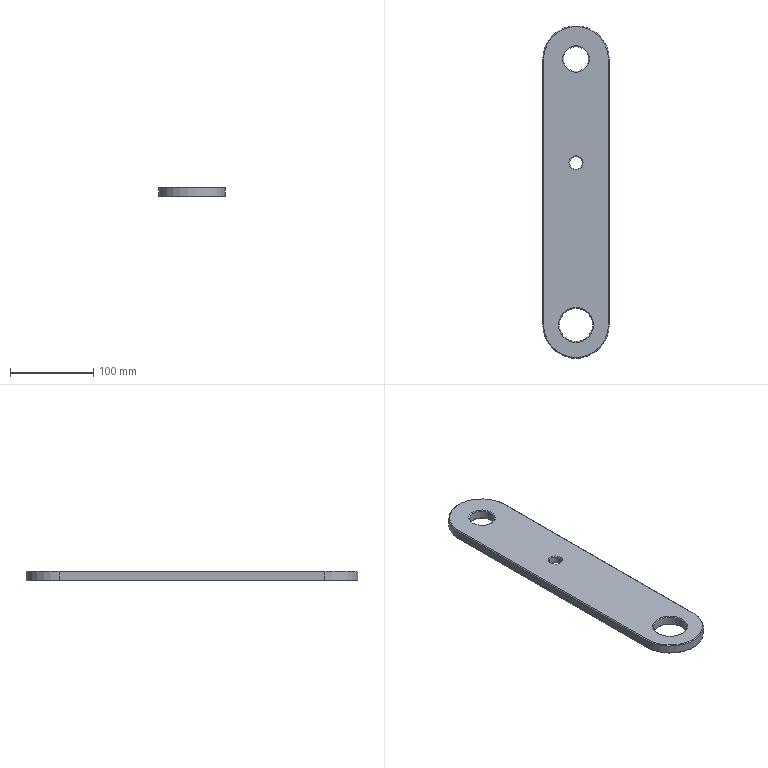Part | SolidWorks | features BaseBody 1 | 1 solid | 35 faces | box 80 x 400 x 12 mm | volume 339060 mm3 | cone 16 | cylinder 10 | plane 9 | commonest cylinder face diameters 30 x4 15 x2 40 x2 80 x2
STEP:
#1=CARTESIAN_POINT('',(-20.,-320.,11.));
#2=VERTEX_POINT('',#1);
#3=CARTESIAN_POINT('',(-21.,-320.,12.));
#4=VERTEX_POINT('',#3);
#5=CARTESIAN_POINT('',(-20.,-320.,11.));
#6=DIRECTION('',(-0.7071,0.,0.7071));
#7=VECTOR('',#6,1000.);
#8=LINE('',#5,#7);
#9=EDGE_CURVE('',#2,#4,#8,.T.);
#10=ORIENTED_EDGE('',*,*,#9,.F.);
#11=CARTESIAN_POINT('',(20.,-320.,11.));
#12=VERTEX_POINT('',#11);
#13=CARTESIAN_POINT('',(0.,-320.,11.));
#14=DIRECTION('',(0.,0.,1.));
#15=DIRECTION('',(1.,0.,0.));
#16=AXIS2_PLACEMENT_3D('',#13,#14,#15);
#17=CIRCLE('',#16,20.);
#18=EDGE_CURVE('',#12,#2,#17,.T.);
#19=ORIENTED_EDGE('',*,*,#18,.F.);
#20=CARTESIAN_POINT('',(21.,-320.,12.));
#21=VERTEX_POINT('',#20);
#22=CARTESIAN_POINT('',(20.,-320.,11.));
#23=DIRECTION('',(0.7071,0.,0.7071));
#24=VECTOR('',#23,1000.);
#25=LINE('',#22,#24);
#26=EDGE_CURVE('',#12,#21,#25,.T.);
#27=ORIENTED_EDGE('',*,*,#26,.T.);
#28=CARTESIAN_POINT('',(0.,-320.,12.));
#29=DIRECTION('',(0.,0.,-1.));
#30=DIRECTION('',(1.,0.,0.));
#31=AXIS2_PLACEMENT_3D('',#28,#29,#30);
#32=CIRCLE('',#31,21.);
#33=EDGE_CURVE('',#4,#21,#32,.T.);
#34=ORIENTED_EDGE('',*,*,#33,.F.);
#35=EDGE_LOOP('',(#10,#19,#27,#34));
#36=FACE_OUTER_BOUND('',#35,.T.);
#37=CARTESIAN_POINT('',(0.,-320.,11.));
#38=DIRECTION('',(0.,0.,1.));
#39=DIRECTION('',(1.,0.,0.));
#40=AXIS2_PLACEMENT_3D('',#37,#38,#39);
#41=CONICAL_SURFACE('',#40,20.,0.7854);
#42=ADVANCED_FACE('',(#36),#41,.F.);
#43=CARTESIAN_POINT('',(39.,-320.,12.));
#44=VERTEX_POINT('',#43);
#45=CARTESIAN_POINT('',(40.,-320.,11.));
#46=VERTEX_POINT('',#45);
#47=CARTESIAN_POINT('',(39.,-320.,12.));
#48=DIRECTION('',(0.7071,0.,-0.7071));
#49=VECTOR('',#48,1000.);
#50=LINE('',#47,#49);
#51=EDGE_CURVE('',#44,#46,#50,.T.);
#52=ORIENTED_EDGE('',*,*,#51,.T.);
#53=CARTESIAN_POINT('',(40.,0.,11.));
#54=VERTEX_POINT('',#53);
#55=CARTESIAN_POINT('',(40.,-320.,11.));
#56=DIRECTION('',(0.,-1.,0.));
#57=VECTOR('',#56,1000.);
#58=LINE('',#55,#57);
#59=EDGE_CURVE('',#54,#46,#58,.T.);
#60=ORIENTED_EDGE('',*,*,#59,.F.);
#61=CARTESIAN_POINT('',(39.,0.,12.));
#62=VERTEX_POINT('',#61);
#63=CARTESIAN_POINT('',(40.,0.,11.));
#64=DIRECTION('',(-0.7071,0.,0.7071));
#65=VECTOR('',#64,1000.);
#66=LINE('',#63,#65);
#67=EDGE_CURVE('',#54,#62,#66,.T.);
#68=ORIENTED_EDGE('',*,*,#67,.T.);
#69=CARTESIAN_POINT('',(39.,0.,12.));
#70=DIRECTION('',(0.,1.,0.));
#71=VECTOR('',#70,1000.);
#72=LINE('',#69,#71);
#73=EDGE_CURVE('',#44,#62,#72,.T.);
#74=ORIENTED_EDGE('',*,*,#73,.F.);
#75=EDGE_LOOP('',(#52,#60,#68,#74));
#76=FACE_OUTER_BOUND('',#75,.T.);
#77=CARTESIAN_POINT('',(39.,0.,12.));
#78=DIRECTION('',(0.7071,0.,0.7071));
#79=DIRECTION('',(0.,-1.,0.));
#80=AXIS2_PLACEMENT_3D('',#77,#78,#79);
#81=PLANE('',#80);
#82=ADVANCED_FACE('',(#76),#81,.T.);
#83=CARTESIAN_POINT('',(-40.,0.,11.));
#84=VERTEX_POINT('',#83);
#85=CARTESIAN_POINT('',(-39.,0.,12.));
#86=VERTEX_POINT('',#85);
#87=CARTESIAN_POINT('',(-40.,0.,11.));
#88=DIRECTION('',(0.7071,0.,0.7071));
#89=VECTOR('',#88,1000.);
#90=LINE('',#87,#89);
#91=EDGE_CURVE('',#84,#86,#90,.T.);
#92=ORIENTED_EDGE('',*,*,#91,.T.);
#93=CARTESIAN_POINT('',(0.,0.,12.));
#94=DIRECTION('',(0.,0.,1.));
#95=DIRECTION('',(1.,0.,0.));
#96=AXIS2_PLACEMENT_3D('',#93,#94,#95);
#97=CIRCLE('',#96,39.);
#98=EDGE_CURVE('',#62,#86,#97,.T.);
#99=ORIENTED_EDGE('',*,*,#98,.F.);
#100=ORIENTED_EDGE('',*,*,#67,.F.);
#101=CARTESIAN_POINT('',(0.,0.,11.));
#102=DIRECTION('',(0.,0.,-1.));
#103=DIRECTION('',(1.,0.,0.));
#104=AXIS2_PLACEMENT_3D('',#101,#102,#103);
#105=CIRCLE('',#104,40.);
#106=EDGE_CURVE('',#84,#54,#105,.T.);
#107=ORIENTED_EDGE('',*,*,#106,.F.);
#108=EDGE_LOOP('',(#92,#99,#100,#107));
#109=FACE_OUTER_BOUND('',#108,.T.);
#110=CARTESIAN_POINT('',(0.,0.,12.));
#111=DIRECTION('',(0.,0.,-1.));
#112=DIRECTION('',(-1.,0.,0.));
#113=AXIS2_PLACEMENT_3D('',#110,#111,#112);
#114=CONICAL_SURFACE('',#113,39.,0.7854);
#115=ADVANCED_FACE('',(#109),#114,.T.);
#116=CARTESIAN_POINT('',(-39.,-320.,12.));
#117=VERTEX_POINT('',#116);
#118=CARTESIAN_POINT('',(-40.,-320.,11.));
#119=VERTEX_POINT('',#118);
#120=CARTESIAN_POINT('',(-39.,-320.,12.));
#121=DIRECTION('',(-0.7071,0.,-0.7071));
#122=VECTOR('',#121,1000.);
#123=LINE('',#120,#122);
#124=EDGE_CURVE('',#117,#119,#123,.T.);
#125=ORIENTED_EDGE('',*,*,#124,.T.);
#126=CARTESIAN_POINT('',(0.,-320.,11.));
#127=DIRECTION('',(0.,0.,-1.));
#128=DIRECTION('',(1.,0.,0.));
#129=AXIS2_PLACEMENT_3D('',#126,#127,#128);
#130=CIRCLE('',#129,40.);
#131=EDGE_CURVE('',#46,#119,#130,.T.);
#132=ORIENTED_EDGE('',*,*,#131,.F.);
#133=ORIENTED_EDGE('',*,*,#51,.F.);
#134=CARTESIAN_POINT('',(0.,-320.,12.));
#135=DIRECTION('',(0.,0.,1.));
#136=DIRECTION('',(1.,0.,0.));
#137=AXIS2_PLACEMENT_3D('',#134,#135,#136);
#138=CIRCLE('',#137,39.);
#139=EDGE_CURVE('',#117,#44,#138,.T.);
#140=ORIENTED_EDGE('',*,*,#139,.F.);
#141=EDGE_LOOP('',(#125,#132,#133,#140));
#142=FACE_OUTER_BOUND('',#141,.T.);
#143=CARTESIAN_POINT('',(0.,-320.,12.));
#144=DIRECTION('',(0.,0.,-1.));
#145=DIRECTION('',(-1.,0.,0.));
#146=AXIS2_PLACEMENT_3D('',#143,#144,#145);
#147=CONICAL_SURFACE('',#146,39.,0.7854);
#148=ADVANCED_FACE('',(#142),#147,.T.);
#149=ORIENTED_EDGE('',*,*,#91,.F.);
#150=CARTESIAN_POINT('',(-40.,0.,11.));
#151=DIRECTION('',(0.,1.,0.));
#152=VECTOR('',#151,1000.);
#153=LINE('',#150,#152);
#154=EDGE_CURVE('',#119,#84,#153,.T.);
#155=ORIENTED_EDGE('',*,*,#154,.F.);
#156=ORIENTED_EDGE('',*,*,#124,.F.);
#157=CARTESIAN_POINT('',(-39.,-320.,12.));
#158=DIRECTION('',(0.,-1.,0.));
#159=VECTOR('',#158,1000.);
#160=LINE('',#157,#159);
#161=EDGE_CURVE('',#86,#117,#160,.T.);
#162=ORIENTED_EDGE('',*,*,#161,.F.);
#163=EDGE_LOOP('',(#149,#155,#156,#162));
#164=FACE_OUTER_BOUND('',#163,.T.);
#165=CARTESIAN_POINT('',(-39.,0.,12.));
#166=DIRECTION('',(-0.7071,0.,0.7071));
#167=DIRECTION('',(0.,1.,0.));
#168=AXIS2_PLACEMENT_3D('',#165,#166,#167);
#169=PLANE('',#168);
#170=ADVANCED_FACE('',(#164),#169,.T.);
#171=CARTESIAN_POINT('',(-15.,0.,11.));
#172=VERTEX_POINT('',#171);
#173=CARTESIAN_POINT('',(-16.,0.,12.));
#174=VERTEX_POINT('',#173);
#175=CARTESIAN_POINT('',(-15.,0.,11.));
#176=DIRECTION('',(-0.7071,0.,0.7071));
#177=VECTOR('',#176,1000.);
#178=LINE('',#175,#177);
#179=EDGE_CURVE('',#172,#174,#178,.T.);
#180=ORIENTED_EDGE('',*,*,#179,.F.);
#181=CARTESIAN_POINT('',(15.,0.,11.));
#182=VERTEX_POINT('',#181);
#183=CARTESIAN_POINT('',(0.,0.,11.));
#184=DIRECTION('',(0.,0.,1.));
#185=DIRECTION('',(1.,0.,0.));
#186=AXIS2_PLACEMENT_3D('',#183,#184,#185);
#187=CIRCLE('',#186,15.);
#188=EDGE_CURVE('',#182,#172,#187,.T.);
#189=ORIENTED_EDGE('',*,*,#188,.F.);
#190=CARTESIAN_POINT('',(16.,0.,12.));
#191=VERTEX_POINT('',#190);
#192=CARTESIAN_POINT('',(15.,0.,11.));
#193=DIRECTION('',(0.7071,0.,0.7071));
#194=VECTOR('',#193,1000.);
#195=LINE('',#192,#194);
#196=EDGE_CURVE('',#182,#191,#195,.T.);
#197=ORIENTED_EDGE('',*,*,#196,.T.);
#198=CARTESIAN_POINT('',(0.,0.,12.));
#199=DIRECTION('',(0.,0.,-1.));
#200=DIRECTION('',(1.,0.,0.));
#201=AXIS2_PLACEMENT_3D('',#198,#199,#200);
#202=CIRCLE('',#201,16.);
#203=EDGE_CURVE('',#174,#191,#202,.T.);
#204=ORIENTED_EDGE('',*,*,#203,.F.);
#205=EDGE_LOOP('',(#180,#189,#197,#204));
#206=FACE_OUTER_BOUND('',#205,.T.);
#207=CARTESIAN_POINT('',(0.,0.,11.));
#208=DIRECTION('',(0.,0.,1.));
#209=DIRECTION('',(1.,0.,0.));
#210=AXIS2_PLACEMENT_3D('',#207,#208,#209);
#211=CONICAL_SURFACE('',#210,15.,0.7854);
#212=ADVANCED_FACE('',(#206),#211,.F.);
#213=CARTESIAN_POINT('',(-7.5,-125.,11.));
#214=VERTEX_POINT('',#213);
#215=CARTESIAN_POINT('',(-8.5,-125.,12.));
#216=VERTEX_POINT('',#215);
#217=CARTESIAN_POINT('',(-7.5,-125.,11.));
#218=DIRECTION('',(-0.7071,0.,0.7071));
#219=VECTOR('',#218,1000.);
#220=LINE('',#217,#219);
#221=EDGE_CURVE('',#214,#216,#220,.T.);
#222=ORIENTED_EDGE('',*,*,#221,.F.);
#223=CARTESIAN_POINT('',(7.5,-125.,11.));
#224=VERTEX_POINT('',#223);
#225=CARTESIAN_POINT('',(0.,-125.,11.));
#226=DIRECTION('',(0.,0.,1.));
#227=DIRECTION('',(1.,0.,0.));
#228=AXIS2_PLACEMENT_3D('',#225,#226,#227);
#229=CIRCLE('',#228,7.5);
#230=EDGE_CURVE('',#224,#214,#229,.T.);
#231=ORIENTED_EDGE('',*,*,#230,.F.);
#232=CARTESIAN_POINT('',(8.5,-125.,12.));
#233=VERTEX_POINT('',#232);
#234=CARTESIAN_POINT('',(7.5,-125.,11.));
#235=DIRECTION('',(0.7071,0.,0.7071));
#236=VECTOR('',#235,1000.);
#237=LINE('',#234,#236);
#238=EDGE_CURVE('',#224,#233,#237,.T.);
#239=ORIENTED_EDGE('',*,*,#238,.T.);
#240=CARTESIAN_POINT('',(0.,-125.,12.));
#241=DIRECTION('',(0.,0.,-1.));
#242=DIRECTION('',(1.,0.,0.));
#243=AXIS2_PLACEMENT_3D('',#240,#241,#242);
#244=CIRCLE('',#243,8.5);
#245=EDGE_CURVE('',#216,#233,#244,.T.);
#246=ORIENTED_EDGE('',*,*,#245,.F.);
#247=EDGE_LOOP('',(#222,#231,#239,#246));
#248=FACE_OUTER_BOUND('',#247,.T.);
#249=CARTESIAN_POINT('',(0.,-125.,11.));
#250=DIRECTION('',(0.,0.,1.));
#251=DIRECTION('',(1.,0.,0.));
#252=AXIS2_PLACEMENT_3D('',#249,#250,#251);
#253=CONICAL_SURFACE('',#252,7.5,0.7854);
#254=ADVANCED_FACE('',(#248),#253,.F.);
#255=CARTESIAN_POINT('',(15.,-125.,1.));
#256=VERTEX_POINT('',#255);
#257=CARTESIAN_POINT('',(16.,-125.,0.));
#258=VERTEX_POINT('',#257);
#259=CARTESIAN_POINT('',(16.,-125.,0.));
#260=DIRECTION('',(0.7071,0.,-0.7071));
#261=VECTOR('',#260,1000.);
#262=LINE('',#259,#261);
#263=EDGE_CURVE('',#256,#258,#262,.T.);
#264=ORIENTED_EDGE('',*,*,#263,.F.);
#265=CARTESIAN_POINT('',(-15.,-125.,1.));
#266=VERTEX_POINT('',#265);
#267=CARTESIAN_POINT('',(0.,-125.,1.));
#268=DIRECTION('',(0.,0.,-1.));
#269=DIRECTION('',(1.,0.,0.));
#270=AXIS2_PLACEMENT_3D('',#267,#268,#269);
#271=CIRCLE('',#270,15.);
#272=EDGE_CURVE('',#266,#256,#271,.T.);
#273=ORIENTED_EDGE('',*,*,#272,.F.);
#274=CARTESIAN_POINT('',(-16.,-125.,0.));
#275=VERTEX_POINT('',#274);
#276=CARTESIAN_POINT('',(-16.,-125.,0.));
#277=DIRECTION('',(-0.7071,0.,-0.7071));
#278=VECTOR('',#277,1000.);
#279=LINE('',#276,#278);
#280=EDGE_CURVE('',#266,#275,#279,.T.);
#281=ORIENTED_EDGE('',*,*,#280,.T.);
#282=CARTESIAN_POINT('',(0.,-125.,0.));
#283=DIRECTION('',(0.,0.,1.));
#284=DIRECTION('',(1.,0.,0.));
#285=AXIS2_PLACEMENT_3D('',#282,#283,#284);
#286=CIRCLE('',#285,16.);
#287=EDGE_CURVE('',#258,#275,#286,.T.);
#288=ORIENTED_EDGE('',*,*,#287,.F.);
#289=EDGE_LOOP('',(#264,#273,#281,#288));
#290=FACE_OUTER_BOUND('',#289,.T.);
#291=CARTESIAN_POINT('',(0.,-125.,0.));
#292=DIRECTION('',(0.,0.,-1.));
#293=DIRECTION('',(-1.,0.,0.));
#294=AXIS2_PLACEMENT_3D('',#291,#292,#293);
#295=CONICAL_SURFACE('',#294,16.,0.7854);
#296=ADVANCED_FACE('',(#290),#295,.F.);
#297=CARTESIAN_POINT('',(-40.,0.,1.));
#298=VERTEX_POINT('',#297);
#299=CARTESIAN_POINT('',(-39.,0.,0.));
#300=VERTEX_POINT('',#299);
#301=CARTESIAN_POINT('',(-40.,0.,1.));
#302=DIRECTION('',(0.7071,0.,-0.7071));
#303=VECTOR('',#302,1000.);
#304=LINE('',#301,#303);
#305=EDGE_CURVE('',#298,#300,#304,.T.);
#306=ORIENTED_EDGE('',*,*,#305,.T.);
#307=CARTESIAN_POINT('',(-39.,-320.,0.));
#308=VERTEX_POINT('',#307);
#309=CARTESIAN_POINT('',(-39.,0.,0.));
#310=DIRECTION('',(0.,1.,0.));
#311=VECTOR('',#310,1000.);
#312=LINE('',#309,#311);
#313=EDGE_CURVE('',#308,#300,#312,.T.);
#314=ORIENTED_EDGE('',*,*,#313,.F.);
#315=CARTESIAN_POINT('',(-40.,-320.,1.));
#316=VERTEX_POINT('',#315);
#317=CARTESIAN_POINT('',(-39.,-320.,0.));
#318=DIRECTION('',(-0.7071,0.,0.7071));
#319=VECTOR('',#318,1000.);
#320=LINE('',#317,#319);
#321=EDGE_CURVE('',#308,#316,#320,.T.);
#322=ORIENTED_EDGE('',*,*,#321,.T.);
#323=CARTESIAN_POINT('',(-40.,0.,1.));
#324=DIRECTION('',(0.,-1.,0.));
#325=VECTOR('',#324,1000.);
#326=LINE('',#323,#325);
#327=EDGE_CURVE('',#298,#316,#326,.T.);
#328=ORIENTED_EDGE('',*,*,#327,.F.);
#329=EDGE_LOOP('',(#306,#314,#322,#328));
#330=FACE_OUTER_BOUND('',#329,.T.);
#331=CARTESIAN_POINT('',(-40.,0.,1.));
#332=DIRECTION('',(0.7071,0.,0.7071));
#333=DIRECTION('',(0.,-1.,0.));
#334=AXIS2_PLACEMENT_3D('',#331,#332,#333);
#335=PLANE('',#334);
#336=ADVANCED_FACE('',(#330),#335,.F.);
#337=CARTESIAN_POINT('',(39.,-320.,0.));
#338=VERTEX_POINT('',#337);
#339=CARTESIAN_POINT('',(40.,-320.,1.));
#340=VERTEX_POINT('',#339);
#341=CARTESIAN_POINT('',(39.,-320.,0.));
#342=DIRECTION('',(0.7071,0.,0.7071));
#343=VECTOR('',#342,1000.);
#344=LINE('',#341,#343);
#345=EDGE_CURVE('',#338,#340,#344,.T.);
#346=ORIENTED_EDGE('',*,*,#345,.T.);
#347=CARTESIAN_POINT('',(0.,-320.,1.));
#348=DIRECTION('',(0.,0.,1.));
#349=DIRECTION('',(1.,0.,0.));
#350=AXIS2_PLACEMENT_3D('',#347,#348,#349);
#351=CIRCLE('',#350,40.);
#352=EDGE_CURVE('',#316,#340,#351,.T.);
#353=ORIENTED_EDGE('',*,*,#352,.F.);
#354=ORIENTED_EDGE('',*,*,#321,.F.);
#355=CARTESIAN_POINT('',(0.,-320.,0.));
#356=DIRECTION('',(0.,0.,-1.));
#357=DIRECTION('',(1.,0.,0.));
#358=AXIS2_PLACEMENT_3D('',#355,#356,#357);
#359=CIRCLE('',#358,39.);
#360=EDGE_CURVE('',#338,#308,#359,.T.);
#361=ORIENTED_EDGE('',*,*,#360,.F.);
#362=EDGE_LOOP('',(#346,#353,#354,#361));
#363=FACE_OUTER_BOUND('',#362,.T.);
#364=CARTESIAN_POINT('',(0.,-320.,1.));
#365=DIRECTION('',(0.,0.,1.));
#366=DIRECTION('',(1.,0.,0.));
#367=AXIS2_PLACEMENT_3D('',#364,#365,#366);
#368=CONICAL_SURFACE('',#367,40.,0.7854);
#369=ADVANCED_FACE('',(#363),#368,.T.);
#370=CARTESIAN_POINT('',(40.,0.,1.));
#371=VERTEX_POINT('',#370);
#372=CARTESIAN_POINT('',(39.,0.,0.));
#373=VERTEX_POINT('',#372);
#374=CARTESIAN_POINT('',(40.,0.,1.));
#375=DIRECTION('',(-0.7071,0.,-0.7071));
#376=VECTOR('',#375,1000.);
#377=LINE('',#374,#376);
#378=EDGE_CURVE('',#371,#373,#377,.T.);
#379=ORIENTED_EDGE('',*,*,#378,.T.);
#380=CARTESIAN_POINT('',(0.,0.,0.));
#381=DIRECTION('',(0.,0.,-1.));
#382=DIRECTION('',(1.,0.,0.));
#383=AXIS2_PLACEMENT_3D('',#380,#381,#382);
#384=CIRCLE('',#383,39.);
#385=EDGE_CURVE('',#300,#373,#384,.T.);
#386=ORIENTED_EDGE('',*,*,#385,.F.);
#387=ORIENTED_EDGE('',*,*,#305,.F.);
#388=CARTESIAN_POINT('',(0.,0.,1.));
#389=DIRECTION('',(0.,0.,1.));
#390=DIRECTION('',(1.,0.,0.));
#391=AXIS2_PLACEMENT_3D('',#388,#389,#390);
#392=CIRCLE('',#391,40.);
#393=EDGE_CURVE('',#371,#298,#392,.T.);
#394=ORIENTED_EDGE('',*,*,#393,.F.);
#395=EDGE_LOOP('',(#379,#386,#387,#394));
#396=FACE_OUTER_BOUND('',#395,.T.);
#397=CARTESIAN_POINT('',(0.,0.,1.));
#398=DIRECTION('',(0.,0.,1.));
#399=DIRECTION('',(1.,0.,0.));
#400=AXIS2_PLACEMENT_3D('',#397,#398,#399);
#401=CONICAL_SURFACE('',#400,40.,0.7854);
#402=ADVANCED_FACE('',(#396),#401,.T.);
#403=ORIENTED_EDGE('',*,*,#345,.F.);
#404=CARTESIAN_POINT('',(39.,0.,0.));
#405=DIRECTION('',(0.,-1.,0.));
#406=VECTOR('',#405,1000.);
#407=LINE('',#404,#406);
#408=EDGE_CURVE('',#373,#338,#407,.T.);
#409=ORIENTED_EDGE('',*,*,#408,.F.);
#410=ORIENTED_EDGE('',*,*,#378,.F.);
#411=CARTESIAN_POINT('',(40.,0.,1.));
#412=DIRECTION('',(0.,1.,0.));
#413=VECTOR('',#412,1000.);
#414=LINE('',#411,#413);
#415=EDGE_CURVE('',#340,#371,#414,.T.);
#416=ORIENTED_EDGE('',*,*,#415,.F.);
#417=EDGE_LOOP('',(#403,#409,#410,#416));
#418=FACE_OUTER_BOUND('',#417,.T.);
#419=CARTESIAN_POINT('',(40.,0.,1.));
#420=DIRECTION('',(-0.7071,0.,0.7071));
#421=DIRECTION('',(0.,1.,0.));
#422=AXIS2_PLACEMENT_3D('',#419,#420,#421);
#423=PLANE('',#422);
#424=ADVANCED_FACE('',(#418),#423,.F.);
#425=CARTESIAN_POINT('',(15.,0.,1.));
#426=VERTEX_POINT('',#425);
#427=CARTESIAN_POINT('',(16.,0.,0.));
#428=VERTEX_POINT('',#427);
#429=CARTESIAN_POINT('',(16.,0.,0.));
#430=DIRECTION('',(0.7071,0.,-0.7071));
#431=VECTOR('',#430,1000.);
#432=LINE('',#429,#431);
#433=EDGE_CURVE('',#426,#428,#432,.T.);
#434=ORIENTED_EDGE('',*,*,#433,.F.);
#435=CARTESIAN_POINT('',(-15.,0.,1.));
#436=VERTEX_POINT('',#435);
#437=CARTESIAN_POINT('',(0.,0.,1.));
#438=DIRECTION('',(0.,0.,-1.));
#439=DIRECTION('',(1.,0.,0.));
#440=AXIS2_PLACEMENT_3D('',#437,#438,#439);
#441=CIRCLE('',#440,15.);
#442=EDGE_CURVE('',#436,#426,#441,.T.);
#443=ORIENTED_EDGE('',*,*,#442,.F.);
#444=CARTESIAN_POINT('',(-16.,0.,0.));
#445=VERTEX_POINT('',#444);
#446=CARTESIAN_POINT('',(-16.,0.,0.));
#447=DIRECTION('',(-0.7071,0.,-0.7071));
#448=VECTOR('',#447,1000.);
#449=LINE('',#446,#448);
#450=EDGE_CURVE('',#436,#445,#449,.T.);
#451=ORIENTED_EDGE('',*,*,#450,.T.);
#452=CARTESIAN_POINT('',(0.,0.,0.));
#453=DIRECTION('',(0.,0.,1.));
#454=DIRECTION('',(1.,0.,0.));
#455=AXIS2_PLACEMENT_3D('',#452,#453,#454);
#456=CIRCLE('',#455,16.);
#457=EDGE_CURVE('',#428,#445,#456,.T.);
#458=ORIENTED_EDGE('',*,*,#457,.F.);
#459=EDGE_LOOP('',(#434,#443,#451,#458));
#460=FACE_OUTER_BOUND('',#459,.T.);
#461=CARTESIAN_POINT('',(0.,0.,0.));
#462=DIRECTION('',(0.,0.,-1.));
#463=DIRECTION('',(-1.,0.,0.));
#464=AXIS2_PLACEMENT_3D('',#461,#462,#463);
#465=CONICAL_SURFACE('',#464,16.,0.7854);
#466=ADVANCED_FACE('',(#460),#465,.F.);
#467=CARTESIAN_POINT('',(20.,-320.,1.));
#468=VERTEX_POINT('',#467);
#469=CARTESIAN_POINT('',(21.,-320.,0.));
#470=VERTEX_POINT('',#469);
#471=CARTESIAN_POINT('',(21.,-320.,0.));
#472=DIRECTION('',(0.7071,0.,-0.7071));
#473=VECTOR('',#472,1000.);
#474=LINE('',#471,#473);
#475=EDGE_CURVE('',#468,#470,#474,.T.);
#476=ORIENTED_EDGE('',*,*,#475,.F.);
#477=CARTESIAN_POINT('',(-20.,-320.,1.));
#478=VERTEX_POINT('',#477);
#479=CARTESIAN_POINT('',(0.,-320.,1.));
#480=DIRECTION('',(0.,0.,-1.));
#481=DIRECTION('',(1.,0.,0.));
#482=AXIS2_PLACEMENT_3D('',#479,#480,#481);
#483=CIRCLE('',#482,20.);
#484=EDGE_CURVE('',#478,#468,#483,.T.);
#485=ORIENTED_EDGE('',*,*,#484,.F.);
#486=CARTESIAN_POINT('',(-21.,-320.,0.));
#487=VERTEX_POINT('',#486);
#488=CARTESIAN_POINT('',(-21.,-320.,0.));
#489=DIRECTION('',(-0.7071,0.,-0.7071));
#490=VECTOR('',#489,1000.);
#491=LINE('',#488,#490);
#492=EDGE_CURVE('',#478,#487,#491,.T.);
#493=ORIENTED_EDGE('',*,*,#492,.T.);
#494=CARTESIAN_POINT('',(0.,-320.,0.));
#495=DIRECTION('',(0.,0.,1.));
#496=DIRECTION('',(1.,0.,0.));
#497=AXIS2_PLACEMENT_3D('',#494,#495,#496);
#498=CIRCLE('',#497,21.);
#499=EDGE_CURVE('',#470,#487,#498,.T.);
#500=ORIENTED_EDGE('',*,*,#499,.F.);
#501=EDGE_LOOP('',(#476,#485,#493,#500));
#502=FACE_OUTER_BOUND('',#501,.T.);
#503=CARTESIAN_POINT('',(0.,-320.,0.));
#504=DIRECTION('',(0.,0.,-1.));
#505=DIRECTION('',(-1.,0.,0.));
#506=AXIS2_PLACEMENT_3D('',#503,#504,#505);
#507=CONICAL_SURFACE('',#506,21.,0.7854);
#508=ADVANCED_FACE('',(#502),#507,.F.);
#509=CARTESIAN_POINT('',(-7.5,-125.,3.));
#510=VERTEX_POINT('',#509);
#511=CARTESIAN_POINT('',(7.5,-125.,3.));
#512=VERTEX_POINT('',#511);
#513=CARTESIAN_POINT('',(0.,-125.,3.));
#514=DIRECTION('',(0.,0.,1.));
#515=DIRECTION('',(1.,0.,0.));
#516=AXIS2_PLACEMENT_3D('',#513,#514,#515);
#517=CIRCLE('',#516,7.5);
#518=EDGE_CURVE('',#510,#512,#517,.T.);
#519=ORIENTED_EDGE('',*,*,#518,.T.);
#520=CARTESIAN_POINT('',(0.,-125.,3.));
#521=DIRECTION('',(0.,0.,1.));
#522=DIRECTION('',(1.,0.,0.));
#523=AXIS2_PLACEMENT_3D('',#520,#521,#522);
#524=CIRCLE('',#523,7.5);
#525=EDGE_CURVE('',#512,#510,#524,.T.);
#526=ORIENTED_EDGE('',*,*,#525,.T.);
#527=EDGE_LOOP('',(#519,#526));
#528=FACE_BOUND('',#527,.T.);
#529=CARTESIAN_POINT('',(-15.,-125.,3.));
#530=VERTEX_POINT('',#529);
#531=CARTESIAN_POINT('',(15.,-125.,3.));
#532=VERTEX_POINT('',#531);
#533=CARTESIAN_POINT('',(0.,-125.,3.));
#534=DIRECTION('',(0.,0.,1.));
#535=DIRECTION('',(1.,0.,0.));
#536=AXIS2_PLACEMENT_3D('',#533,#534,#535);
#537=CIRCLE('',#536,15.);
#538=EDGE_CURVE('',#530,#532,#537,.T.);
#539=ORIENTED_EDGE('',*,*,#538,.F.);
#540=CARTESIAN_POINT('',(0.,-125.,3.));
#541=DIRECTION('',(0.,0.,1.));
#542=DIRECTION('',(1.,0.,0.));
#543=AXIS2_PLACEMENT_3D('',#540,#541,#542);
#544=CIRCLE('',#543,15.);
#545=EDGE_CURVE('',#532,#530,#544,.T.);
#546=ORIENTED_EDGE('',*,*,#545,.F.);
#547=EDGE_LOOP('',(#539,#546));
#548=FACE_OUTER_BOUND('',#547,.T.);
#549=CARTESIAN_POINT('',(0.,-125.,3.));
#550=DIRECTION('',(0.,0.,1.));
#551=DIRECTION('',(1.,0.,0.));
#552=AXIS2_PLACEMENT_3D('',#549,#550,#551);
#553=PLANE('',#552);
#554=ADVANCED_FACE('',(#528,#548),#553,.F.);
#555=CARTESIAN_POINT('',(15.,-125.,3.));
#556=DIRECTION('',(0.,0.,-1.));
#557=VECTOR('',#556,1000.);
#558=LINE('',#555,#557);
#559=EDGE_CURVE('',#532,#256,#558,.T.);
#560=ORIENTED_EDGE('',*,*,#559,.F.);
#561=ORIENTED_EDGE('',*,*,#545,.T.);
#562=CARTESIAN_POINT('',(-15.,-125.,3.));
#563=DIRECTION('',(0.,0.,-1.));
#564=VECTOR('',#563,1000.);
#565=LINE('',#562,#564);
#566=EDGE_CURVE('',#530,#266,#565,.T.);
#567=ORIENTED_EDGE('',*,*,#566,.T.);
#568=ORIENTED_EDGE('',*,*,#272,.T.);
#569=EDGE_LOOP('',(#560,#561,#567,#568));
#570=FACE_OUTER_BOUND('',#569,.T.);
#571=CARTESIAN_POINT('',(0.,-125.,3.));
#572=DIRECTION('',(0.,0.,-1.));
#573=DIRECTION('',(-1.,0.,0.));
#574=AXIS2_PLACEMENT_3D('',#571,#572,#573);
#575=CYLINDRICAL_SURFACE('',#574,15.);
#576=ADVANCED_FACE('',(#570),#575,.F.);
#577=CARTESIAN_POINT('',(7.5,-125.,12.));
#578=DIRECTION('',(0.,0.,-1.));
#579=VECTOR('',#578,1000.);
#580=LINE('',#577,#579);
#581=EDGE_CURVE('',#224,#512,#580,.T.);
#582=ORIENTED_EDGE('',*,*,#581,.F.);
#583=ORIENTED_EDGE('',*,*,#230,.T.);
#584=CARTESIAN_POINT('',(-7.5,-125.,12.));
#585=DIRECTION('',(0.,0.,-1.));
#586=VECTOR('',#585,1000.);
#587=LINE('',#584,#586);
#588=EDGE_CURVE('',#214,#510,#587,.T.);
#589=ORIENTED_EDGE('',*,*,#588,.T.);
#590=ORIENTED_EDGE('',*,*,#525,.F.);
#591=EDGE_LOOP('',(#582,#583,#589,#590));
#592=FACE_OUTER_BOUND('',#591,.T.);
#593=CARTESIAN_POINT('',(0.,-125.,12.));
#594=DIRECTION('',(0.,0.,-1.));
#595=DIRECTION('',(-1.,0.,0.));
#596=AXIS2_PLACEMENT_3D('',#593,#594,#595);
#597=CYLINDRICAL_SURFACE('',#596,7.5);
#598=ADVANCED_FACE('',(#592),#597,.F.);
#599=CARTESIAN_POINT('',(20.,-320.,12.));
#600=DIRECTION('',(0.,0.,-1.));
#601=VECTOR('',#600,1000.);
#602=LINE('',#599,#601);
#603=EDGE_CURVE('',#12,#468,#602,.T.);
#604=ORIENTED_EDGE('',*,*,#603,.F.);
#605=ORIENTED_EDGE('',*,*,#18,.T.);
#606=CARTESIAN_POINT('',(-20.,-320.,12.));
#607=DIRECTION('',(0.,0.,-1.));
#608=VECTOR('',#607,1000.);
#609=LINE('',#606,#608);
#610=EDGE_CURVE('',#2,#478,#609,.T.);
#611=ORIENTED_EDGE('',*,*,#610,.T.);
#612=ORIENTED_EDGE('',*,*,#484,.T.);
#613=EDGE_LOOP('',(#604,#605,#611,#612));
#614=FACE_OUTER_BOUND('',#613,.T.);
#615=CARTESIAN_POINT('',(0.,-320.,12.));
#616=DIRECTION('',(0.,0.,-1.));
#617=DIRECTION('',(-1.,0.,0.));
#618=AXIS2_PLACEMENT_3D('',#615,#616,#617);
#619=CYLINDRICAL_SURFACE('',#618,20.);
#620=ADVANCED_FACE('',(#614),#619,.F.);
#621=CARTESIAN_POINT('',(15.,0.,12.));
#622=DIRECTION('',(0.,0.,-1.));
#623=VECTOR('',#622,1000.);
#624=LINE('',#621,#623);
#625=EDGE_CURVE('',#182,#426,#624,.T.);
#626=ORIENTED_EDGE('',*,*,#625,.F.);
#627=ORIENTED_EDGE('',*,*,#188,.T.);
#628=CARTESIAN_POINT('',(-15.,0.,12.));
#629=DIRECTION('',(0.,0.,-1.));
#630=VECTOR('',#629,1000.);
#631=LINE('',#628,#630);
#632=EDGE_CURVE('',#172,#436,#631,.T.);
#633=ORIENTED_EDGE('',*,*,#632,.T.);
#634=ORIENTED_EDGE('',*,*,#442,.T.);
#635=EDGE_LOOP('',(#626,#627,#633,#634));
#636=FACE_OUTER_BOUND('',#635,.T.);
#637=CARTESIAN_POINT('',(0.,0.,12.));
#638=DIRECTION('',(0.,0.,-1.));
#639=DIRECTION('',(-1.,0.,0.));
#640=AXIS2_PLACEMENT_3D('',#637,#638,#639);
#641=CYLINDRICAL_SURFACE('',#640,15.);
#642=ADVANCED_FACE('',(#636),#641,.F.);
#643=CARTESIAN_POINT('',(40.,-320.,12.));
#644=DIRECTION('',(0.,0.,-1.));
#645=VECTOR('',#644,1000.);
#646=LINE('',#643,#645);
#647=EDGE_CURVE('',#46,#340,#646,.T.);
#648=ORIENTED_EDGE('',*,*,#647,.T.);
#649=ORIENTED_EDGE('',*,*,#415,.T.);
#650=CARTESIAN_POINT('',(40.,0.,12.));
#651=DIRECTION('',(0.,0.,-1.));
#652=VECTOR('',#651,1000.);
#653=LINE('',#650,#652);
#654=EDGE_CURVE('',#54,#371,#653,.T.);
#655=ORIENTED_EDGE('',*,*,#654,.F.);
#656=ORIENTED_EDGE('',*,*,#59,.T.);
#657=EDGE_LOOP('',(#648,#649,#655,#656));
#658=FACE_OUTER_BOUND('',#657,.T.);
#659=CARTESIAN_POINT('',(40.,0.,12.));
#660=DIRECTION('',(-1.,0.,0.));
#661=DIRECTION('',(0.,1.,0.));
#662=AXIS2_PLACEMENT_3D('',#659,#660,#661);
#663=PLANE('',#662);
#664=ADVANCED_FACE('',(#658),#663,.F.);
#665=CARTESIAN_POINT('',(-40.,-320.,12.));
#666=DIRECTION('',(0.,0.,-1.));
#667=VECTOR('',#666,1000.);
#668=LINE('',#665,#667);
#669=EDGE_CURVE('',#119,#316,#668,.T.);
#670=ORIENTED_EDGE('',*,*,#669,.T.);
#671=ORIENTED_EDGE('',*,*,#352,.T.);
#672=ORIENTED_EDGE('',*,*,#647,.F.);
#673=ORIENTED_EDGE('',*,*,#131,.T.);
#674=EDGE_LOOP('',(#670,#671,#672,#673));
#675=FACE_OUTER_BOUND('',#674,.T.);
#676=CARTESIAN_POINT('',(0.,-320.,12.));
#677=DIRECTION('',(0.,0.,-1.));
#678=DIRECTION('',(-1.,0.,0.));
#679=AXIS2_PLACEMENT_3D('',#676,#677,#678);
#680=CYLINDRICAL_SURFACE('',#679,40.);
#681=ADVANCED_FACE('',(#675),#680,.T.);
#682=CARTESIAN_POINT('',(-40.,0.,12.));
#683=DIRECTION('',(0.,0.,-1.));
#684=VECTOR('',#683,1000.);
#685=LINE('',#682,#684);
#686=EDGE_CURVE('',#84,#298,#685,.T.);
#687=ORIENTED_EDGE('',*,*,#686,.T.);
#688=ORIENTED_EDGE('',*,*,#327,.T.);
#689=ORIENTED_EDGE('',*,*,#669,.F.);
#690=ORIENTED_EDGE('',*,*,#154,.T.);
#691=EDGE_LOOP('',(#687,#688,#689,#690));
#692=FACE_OUTER_BOUND('',#691,.T.);
#693=CARTESIAN_POINT('',(-40.,0.,12.));
#694=DIRECTION('',(1.,0.,0.));
#695=DIRECTION('',(0.,1.,0.));
#696=AXIS2_PLACEMENT_3D('',#693,#694,#695);
#697=PLANE('',#696);
#698=ADVANCED_FACE('',(#692),#697,.F.);
#699=ORIENTED_EDGE('',*,*,#654,.T.);
#700=ORIENTED_EDGE('',*,*,#393,.T.);
#701=ORIENTED_EDGE('',*,*,#686,.F.);
#702=ORIENTED_EDGE('',*,*,#106,.T.);
#703=EDGE_LOOP('',(#699,#700,#701,#702));
#704=FACE_OUTER_BOUND('',#703,.T.);
#705=CARTESIAN_POINT('',(0.,0.,12.));
#706=DIRECTION('',(0.,0.,-1.));
#707=DIRECTION('',(-1.,0.,0.));
#708=AXIS2_PLACEMENT_3D('',#705,#706,#707);
#709=CYLINDRICAL_SURFACE('',#708,40.);
#710=ADVANCED_FACE('',(#704),#709,.T.);
#711=CARTESIAN_POINT('',(0.,-125.,0.));
#712=DIRECTION('',(0.,0.,1.));
#713=DIRECTION('',(1.,0.,0.));
#714=AXIS2_PLACEMENT_3D('',#711,#712,#713);
#715=CIRCLE('',#714,16.);
#716=EDGE_CURVE('',#275,#258,#715,.T.);
#717=ORIENTED_EDGE('',*,*,#716,.T.);
#718=ORIENTED_EDGE('',*,*,#287,.T.);
#719=EDGE_LOOP('',(#717,#718));
#720=FACE_BOUND('',#719,.T.);
#721=CARTESIAN_POINT('',(0.,0.,0.));
#722=DIRECTION('',(0.,0.,1.));
#723=DIRECTION('',(1.,0.,0.));
#724=AXIS2_PLACEMENT_3D('',#721,#722,#723);
#725=CIRCLE('',#724,16.);
#726=EDGE_CURVE('',#445,#428,#725,.T.);
#727=ORIENTED_EDGE('',*,*,#726,.T.);
#728=ORIENTED_EDGE('',*,*,#457,.T.);
#729=EDGE_LOOP('',(#727,#728));
#730=FACE_BOUND('',#729,.T.);
#731=CARTESIAN_POINT('',(0.,-320.,0.));
#732=DIRECTION('',(0.,0.,1.));
#733=DIRECTION('',(1.,0.,0.));
#734=AXIS2_PLACEMENT_3D('',#731,#732,#733);
#735=CIRCLE('',#734,21.);
#736=EDGE_CURVE('',#487,#470,#735,.T.);
#737=ORIENTED_EDGE('',*,*,#736,.T.);
#738=ORIENTED_EDGE('',*,*,#499,.T.);
#739=EDGE_LOOP('',(#737,#738));
#740=FACE_BOUND('',#739,.T.);
#741=ORIENTED_EDGE('',*,*,#360,.T.);
#742=ORIENTED_EDGE('',*,*,#313,.T.);
#743=ORIENTED_EDGE('',*,*,#385,.T.);
#744=ORIENTED_EDGE('',*,*,#408,.T.);
#745=EDGE_LOOP('',(#741,#742,#743,#744));
#746=FACE_OUTER_BOUND('',#745,.T.);
#747=CARTESIAN_POINT('',(0.,0.,0.));
#748=DIRECTION('',(0.,0.,1.));
#749=DIRECTION('',(1.,0.,0.));
#750=AXIS2_PLACEMENT_3D('',#747,#748,#749);
#751=PLANE('',#750);
#752=ADVANCED_FACE('',(#720,#730,#740,#746),#751,.F.);
#753=CARTESIAN_POINT('',(0.,-320.,12.));
#754=DIRECTION('',(0.,0.,-1.));
#755=DIRECTION('',(1.,0.,0.));
#756=AXIS2_PLACEMENT_3D('',#753,#754,#755);
#757=CIRCLE('',#756,21.);
#758=EDGE_CURVE('',#21,#4,#757,.T.);
#759=ORIENTED_EDGE('',*,*,#758,.T.);
#760=ORIENTED_EDGE('',*,*,#33,.T.);
#761=EDGE_LOOP('',(#759,#760));
#762=FACE_BOUND('',#761,.T.);
#763=CARTESIAN_POINT('',(0.,0.,12.));
#764=DIRECTION('',(0.,0.,-1.));
#765=DIRECTION('',(1.,0.,0.));
#766=AXIS2_PLACEMENT_3D('',#763,#764,#765);
#767=CIRCLE('',#766,16.);
#768=EDGE_CURVE('',#191,#174,#767,.T.);
#769=ORIENTED_EDGE('',*,*,#768,.T.);
#770=ORIENTED_EDGE('',*,*,#203,.T.);
#771=EDGE_LOOP('',(#769,#770));
#772=FACE_BOUND('',#771,.T.);
#773=CARTESIAN_POINT('',(0.,-125.,12.));
#774=DIRECTION('',(0.,0.,-1.));
#775=DIRECTION('',(1.,0.,0.));
#776=AXIS2_PLACEMENT_3D('',#773,#774,#775);
#777=CIRCLE('',#776,8.5);
#778=EDGE_CURVE('',#233,#216,#777,.T.);
#779=ORIENTED_EDGE('',*,*,#778,.T.);
#780=ORIENTED_EDGE('',*,*,#245,.T.);
#781=EDGE_LOOP('',(#779,#780));
#782=FACE_BOUND('',#781,.T.);
#783=ORIENTED_EDGE('',*,*,#139,.T.);
#784=ORIENTED_EDGE('',*,*,#73,.T.);
#785=ORIENTED_EDGE('',*,*,#98,.T.);
#786=ORIENTED_EDGE('',*,*,#161,.T.);
#787=EDGE_LOOP('',(#783,#784,#785,#786));
#788=FACE_OUTER_BOUND('',#787,.T.);
#789=CARTESIAN_POINT('',(0.,0.,12.));
#790=DIRECTION('',(0.,0.,1.));
#791=DIRECTION('',(1.,0.,0.));
#792=AXIS2_PLACEMENT_3D('',#789,#790,#791);
#793=PLANE('',#792);
#794=ADVANCED_FACE('',(#762,#772,#782,#788),#793,.T.);
#795=CARTESIAN_POINT('',(0.,0.,11.));
#796=DIRECTION('',(0.,0.,1.));
#797=DIRECTION('',(1.,0.,0.));
#798=AXIS2_PLACEMENT_3D('',#795,#796,#797);
#799=CIRCLE('',#798,15.);
#800=EDGE_CURVE('',#172,#182,#799,.T.);
#801=ORIENTED_EDGE('',*,*,#800,.T.);
#802=ORIENTED_EDGE('',*,*,#625,.T.);
#803=CARTESIAN_POINT('',(0.,0.,1.));
#804=DIRECTION('',(0.,0.,-1.));
#805=DIRECTION('',(1.,0.,0.));
#806=AXIS2_PLACEMENT_3D('',#803,#804,#805);
#807=CIRCLE('',#806,15.);
#808=EDGE_CURVE('',#426,#436,#807,.T.);
#809=ORIENTED_EDGE('',*,*,#808,.T.);
#810=ORIENTED_EDGE('',*,*,#632,.F.);
#811=EDGE_LOOP('',(#801,#802,#809,#810));
#812=FACE_OUTER_BOUND('',#811,.T.);
#813=CARTESIAN_POINT('',(0.,0.,12.));
#814=DIRECTION('',(0.,0.,-1.));
#815=DIRECTION('',(-1.,0.,0.));
#816=AXIS2_PLACEMENT_3D('',#813,#814,#815);
#817=CYLINDRICAL_SURFACE('',#816,15.);
#818=ADVANCED_FACE('',(#812),#817,.F.);
#819=CARTESIAN_POINT('',(0.,-320.,11.));
#820=DIRECTION('',(0.,0.,1.));
#821=DIRECTION('',(1.,0.,0.));
#822=AXIS2_PLACEMENT_3D('',#819,#820,#821);
#823=CIRCLE('',#822,20.);
#824=EDGE_CURVE('',#2,#12,#823,.T.);
#825=ORIENTED_EDGE('',*,*,#824,.T.);
#826=ORIENTED_EDGE('',*,*,#603,.T.);
#827=CARTESIAN_POINT('',(0.,-320.,1.));
#828=DIRECTION('',(0.,0.,-1.));
#829=DIRECTION('',(1.,0.,0.));
#830=AXIS2_PLACEMENT_3D('',#827,#828,#829);
#831=CIRCLE('',#830,20.);
#832=EDGE_CURVE('',#468,#478,#831,.T.);
#833=ORIENTED_EDGE('',*,*,#832,.T.);
#834=ORIENTED_EDGE('',*,*,#610,.F.);
#835=EDGE_LOOP('',(#825,#826,#833,#834));
#836=FACE_OUTER_BOUND('',#835,.T.);
#837=CARTESIAN_POINT('',(0.,-320.,12.));
#838=DIRECTION('',(0.,0.,-1.));
#839=DIRECTION('',(-1.,0.,0.));
#840=AXIS2_PLACEMENT_3D('',#837,#838,#839);
#841=CYLINDRICAL_SURFACE('',#840,20.);
#842=ADVANCED_FACE('',(#836),#841,.F.);
#843=CARTESIAN_POINT('',(0.,-125.,11.));
#844=DIRECTION('',(0.,0.,1.));
#845=DIRECTION('',(1.,0.,0.));
#846=AXIS2_PLACEMENT_3D('',#843,#844,#845);
#847=CIRCLE('',#846,7.5);
#848=EDGE_CURVE('',#214,#224,#847,.T.);
#849=ORIENTED_EDGE('',*,*,#848,.T.);
#850=ORIENTED_EDGE('',*,*,#581,.T.);
#851=ORIENTED_EDGE('',*,*,#518,.F.);
#852=ORIENTED_EDGE('',*,*,#588,.F.);
#853=EDGE_LOOP('',(#849,#850,#851,#852));
#854=FACE_OUTER_BOUND('',#853,.T.);
#855=CARTESIAN_POINT('',(0.,-125.,12.));
#856=DIRECTION('',(0.,0.,-1.));
#857=DIRECTION('',(-1.,0.,0.));
#858=AXIS2_PLACEMENT_3D('',#855,#856,#857);
#859=CYLINDRICAL_SURFACE('',#858,7.5);
#860=ADVANCED_FACE('',(#854),#859,.F.);
#861=ORIENTED_EDGE('',*,*,#538,.T.);
#862=ORIENTED_EDGE('',*,*,#559,.T.);
#863=CARTESIAN_POINT('',(0.,-125.,1.));
#864=DIRECTION('',(0.,0.,-1.));
#865=DIRECTION('',(1.,0.,0.));
#866=AXIS2_PLACEMENT_3D('',#863,#864,#865);
#867=CIRCLE('',#866,15.);
#868=EDGE_CURVE('',#256,#266,#867,.T.);
#869=ORIENTED_EDGE('',*,*,#868,.T.);
#870=ORIENTED_EDGE('',*,*,#566,.F.);
#871=EDGE_LOOP('',(#861,#862,#869,#870));
#872=FACE_OUTER_BOUND('',#871,.T.);
#873=CARTESIAN_POINT('',(0.,-125.,3.));
#874=DIRECTION('',(0.,0.,-1.));
#875=DIRECTION('',(-1.,0.,0.));
#876=AXIS2_PLACEMENT_3D('',#873,#874,#875);
#877=CYLINDRICAL_SURFACE('',#876,15.);
#878=ADVANCED_FACE('',(#872),#877,.F.);
#879=ORIENTED_EDGE('',*,*,#832,.F.);
#880=ORIENTED_EDGE('',*,*,#475,.T.);
#881=ORIENTED_EDGE('',*,*,#736,.F.);
#882=ORIENTED_EDGE('',*,*,#492,.F.);
#883=EDGE_LOOP('',(#879,#880,#881,#882));
#884=FACE_OUTER_BOUND('',#883,.T.);
#885=CARTESIAN_POINT('',(0.,-320.,0.));
#886=DIRECTION('',(0.,0.,-1.));
#887=DIRECTION('',(-1.,0.,0.));
#888=AXIS2_PLACEMENT_3D('',#885,#886,#887);
#889=CONICAL_SURFACE('',#888,21.,0.7854);
#890=ADVANCED_FACE('',(#884),#889,.F.);
#891=ORIENTED_EDGE('',*,*,#808,.F.);
#892=ORIENTED_EDGE('',*,*,#433,.T.);
#893=ORIENTED_EDGE('',*,*,#726,.F.);
#894=ORIENTED_EDGE('',*,*,#450,.F.);
#895=EDGE_LOOP('',(#891,#892,#893,#894));
#896=FACE_OUTER_BOUND('',#895,.T.);
#897=CARTESIAN_POINT('',(0.,0.,0.));
#898=DIRECTION('',(0.,0.,-1.));
#899=DIRECTION('',(-1.,0.,0.));
#900=AXIS2_PLACEMENT_3D('',#897,#898,#899);
#901=CONICAL_SURFACE('',#900,16.,0.7854);
#902=ADVANCED_FACE('',(#896),#901,.F.);
#903=ORIENTED_EDGE('',*,*,#868,.F.);
#904=ORIENTED_EDGE('',*,*,#263,.T.);
#905=ORIENTED_EDGE('',*,*,#716,.F.);
#906=ORIENTED_EDGE('',*,*,#280,.F.);
#907=EDGE_LOOP('',(#903,#904,#905,#906));
#908=FACE_OUTER_BOUND('',#907,.T.);
#909=CARTESIAN_POINT('',(0.,-125.,0.));
#910=DIRECTION('',(0.,0.,-1.));
#911=DIRECTION('',(-1.,0.,0.));
#912=AXIS2_PLACEMENT_3D('',#909,#910,#911);
#913=CONICAL_SURFACE('',#912,16.,0.7854);
#914=ADVANCED_FACE('',(#908),#913,.F.);
#915=ORIENTED_EDGE('',*,*,#848,.F.);
#916=ORIENTED_EDGE('',*,*,#221,.T.);
#917=ORIENTED_EDGE('',*,*,#778,.F.);
#918=ORIENTED_EDGE('',*,*,#238,.F.);
#919=EDGE_LOOP('',(#915,#916,#917,#918));
#920=FACE_OUTER_BOUND('',#919,.T.);
#921=CARTESIAN_POINT('',(0.,-125.,11.));
#922=DIRECTION('',(0.,0.,1.));
#923=DIRECTION('',(1.,0.,0.));
#924=AXIS2_PLACEMENT_3D('',#921,#922,#923);
#925=CONICAL_SURFACE('',#924,7.5,0.7854);
#926=ADVANCED_FACE('',(#920),#925,.F.);
#927=ORIENTED_EDGE('',*,*,#800,.F.);
#928=ORIENTED_EDGE('',*,*,#179,.T.);
#929=ORIENTED_EDGE('',*,*,#768,.F.);
#930=ORIENTED_EDGE('',*,*,#196,.F.);
#931=EDGE_LOOP('',(#927,#928,#929,#930));
#932=FACE_OUTER_BOUND('',#931,.T.);
#933=CARTESIAN_POINT('',(0.,0.,11.));
#934=DIRECTION('',(0.,0.,1.));
#935=DIRECTION('',(1.,0.,0.));
#936=AXIS2_PLACEMENT_3D('',#933,#934,#935);
#937=CONICAL_SURFACE('',#936,15.,0.7854);
#938=ADVANCED_FACE('',(#932),#937,.F.);
#939=ORIENTED_EDGE('',*,*,#824,.F.);
#940=ORIENTED_EDGE('',*,*,#9,.T.);
#941=ORIENTED_EDGE('',*,*,#758,.F.);
#942=ORIENTED_EDGE('',*,*,#26,.F.);
#943=EDGE_LOOP('',(#939,#940,#941,#942));
#944=FACE_OUTER_BOUND('',#943,.T.);
#945=CARTESIAN_POINT('',(0.,-320.,11.));
#946=DIRECTION('',(0.,0.,1.));
#947=DIRECTION('',(1.,0.,0.));
#948=AXIS2_PLACEMENT_3D('',#945,#946,#947);
#949=CONICAL_SURFACE('',#948,20.,0.7854);
#950=ADVANCED_FACE('',(#944),#949,.F.);
#951=CLOSED_SHELL('',(#42,#82,#115,#148,#170,#212,#254,#296,#336,#369,#402,#424,#466,#508,#554,#576,#598,#620,#642,#664,#681,#698,#710,#752,#794,#818,#842,#860,#878,#890,#902,#914,#926,#938,#950));
#952=MANIFOLD_SOLID_BREP('',#951);
#953=CARTESIAN_POINT('',(0.,0.,0.));
#954=DIRECTION('',(0.,0.,1.));
#955=DIRECTION('',(1.,0.,0.));
#956=AXIS2_PLACEMENT_3D('',#953,#954,#955);
#957=(LENGTH_UNIT()NAMED_UNIT(*)SI_UNIT(.MILLI.,.METRE.));
#958=UNCERTAINTY_MEASURE_WITH_UNIT(LENGTH_MEASURE(0.00001),#957,'','');
#959=(NAMED_UNIT(*)PLANE_ANGLE_UNIT()SI_UNIT($,.RADIAN.));
#960=(NAMED_UNIT(*)SI_UNIT($,.STERADIAN.)SOLID_ANGLE_UNIT());
#961=(GEOMETRIC_REPRESENTATION_CONTEXT(3)GLOBAL_UNCERTAINTY_ASSIGNED_CONTEXT((#958))GLOBAL_UNIT_ASSIGNED_CONTEXT((#957,#959,#960))REPRESENTATION_CONTEXT('',''));
#962=ADVANCED_BREP_SHAPE_REPRESENTATION('',(#952,#956),#961);